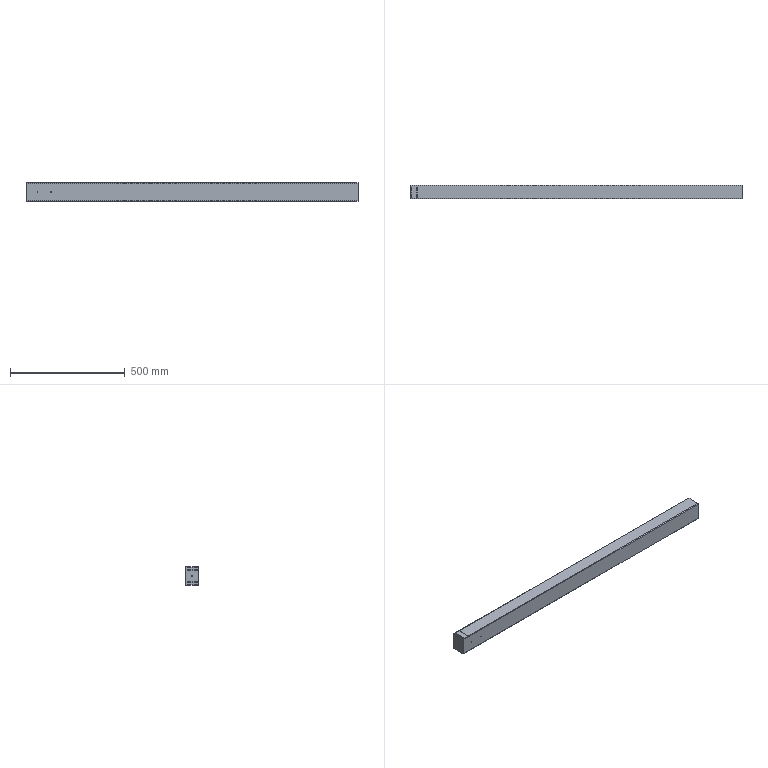Part | NX | 1 solid | 55 faces | box 1446 x 60 x 80 mm | volume 2283808 mm3 | cylinder 33 | plane 12 | cone 10 | commonest cylinder face diameters 3.3 x20 5.236 x8 4.2 x5
STEP:
#1=CARTESIAN_POINT('',(1126.,565.,37.382));
#2=VERTEX_POINT('',#1);
#3=CARTESIAN_POINT('',(-320.,565.,37.382));
#4=VERTEX_POINT('',#3);
#5=CARTESIAN_POINT('',(1126.,565.,37.382));
#6=DIRECTION('',(-1.,0.,0.));
#7=VECTOR('',#6,1000.);
#8=LINE('',#5,#7);
#9=EDGE_CURVE('',#2,#4,#8,.T.);
#10=ORIENTED_EDGE('',*,*,#9,.T.);
#11=CARTESIAN_POINT('',(-320.,562.382,40.));
#12=VERTEX_POINT('',#11);
#13=CARTESIAN_POINT('',(-320.,562.382,37.382));
#14=DIRECTION('',(1.,0.,0.));
#15=DIRECTION('',(0.,0.,1.));
#16=AXIS2_PLACEMENT_3D('',#13,#14,#15);
#17=CIRCLE('',#16,2.618);
#18=EDGE_CURVE('',#4,#12,#17,.T.);
#19=ORIENTED_EDGE('',*,*,#18,.T.);
#20=CARTESIAN_POINT('',(1126.,562.382,40.));
#21=VERTEX_POINT('',#20);
#22=CARTESIAN_POINT('',(1126.,562.382,40.));
#23=DIRECTION('',(-1.,0.,0.));
#24=VECTOR('',#23,1000.);
#25=LINE('',#22,#24);
#26=EDGE_CURVE('',#21,#12,#25,.T.);
#27=ORIENTED_EDGE('',*,*,#26,.F.);
#28=CARTESIAN_POINT('',(1126.,562.382,37.382));
#29=DIRECTION('',(1.,0.,0.));
#30=DIRECTION('',(0.,0.,1.));
#31=AXIS2_PLACEMENT_3D('',#28,#29,#30);
#32=CIRCLE('',#31,2.618);
#33=EDGE_CURVE('',#2,#21,#32,.T.);
#34=ORIENTED_EDGE('',*,*,#33,.F.);
#35=EDGE_LOOP('',(#10,#19,#27,#34));
#36=FACE_BOUND('',#35,.T.);
#37=CARTESIAN_POINT('',(1126.,562.382,37.382));
#38=DIRECTION('',(-1.,0.,0.));
#39=DIRECTION('',(0.,0.,1.));
#40=AXIS2_PLACEMENT_3D('',#37,#38,#39);
#41=CYLINDRICAL_SURFACE('',#40,2.618);
#42=ADVANCED_FACE('',(#36),#41,.T.);
#43=CARTESIAN_POINT('',(-289.5,551.35,40.));
#44=VERTEX_POINT('',#43);
#45=CARTESIAN_POINT('',(-289.5,553.,40.));
#46=DIRECTION('',(0.,0.,1.));
#47=DIRECTION('',(0.,-1.,0.));
#48=AXIS2_PLACEMENT_3D('',#45,#46,#47);
#49=CIRCLE('',#48,1.65);
#50=EDGE_CURVE('',#44,#44,#49,.T.);
#51=ORIENTED_EDGE('',*,*,#50,.F.);
#52=EDGE_LOOP('',(#51));
#53=FACE_BOUND('',#52,.T.);
#54=CARTESIAN_POINT('',(-314.5,551.35,40.));
#55=VERTEX_POINT('',#54);
#56=CARTESIAN_POINT('',(-314.5,553.,40.));
#57=DIRECTION('',(0.,0.,1.));
#58=DIRECTION('',(0.,-1.,0.));
#59=AXIS2_PLACEMENT_3D('',#56,#57,#58);
#60=CIRCLE('',#59,1.65);
#61=EDGE_CURVE('',#55,#55,#60,.T.);
#62=ORIENTED_EDGE('',*,*,#61,.F.);
#63=EDGE_LOOP('',(#62));
#64=FACE_BOUND('',#63,.T.);
#65=CARTESIAN_POINT('',(-289.5,541.35,40.));
#66=VERTEX_POINT('',#65);
#67=CARTESIAN_POINT('',(-289.5,543.,40.));
#68=DIRECTION('',(0.,0.,1.));
#69=DIRECTION('',(0.,-1.,0.));
#70=AXIS2_PLACEMENT_3D('',#67,#68,#69);
#71=CIRCLE('',#70,1.65);
#72=EDGE_CURVE('',#66,#66,#71,.T.);
#73=ORIENTED_EDGE('',*,*,#72,.F.);
#74=EDGE_LOOP('',(#73));
#75=FACE_BOUND('',#74,.T.);
#76=CARTESIAN_POINT('',(-314.5,541.35,40.));
#77=VERTEX_POINT('',#76);
#78=CARTESIAN_POINT('',(-314.5,543.,40.));
#79=DIRECTION('',(0.,0.,1.));
#80=DIRECTION('',(0.,-1.,0.));
#81=AXIS2_PLACEMENT_3D('',#78,#79,#80);
#82=CIRCLE('',#81,1.65);
#83=EDGE_CURVE('',#77,#77,#82,.T.);
#84=ORIENTED_EDGE('',*,*,#83,.F.);
#85=EDGE_LOOP('',(#84));
#86=FACE_BOUND('',#85,.T.);
#87=CARTESIAN_POINT('',(-289.5,531.35,40.));
#88=VERTEX_POINT('',#87);
#89=CARTESIAN_POINT('',(-289.5,533.,40.));
#90=DIRECTION('',(0.,0.,1.));
#91=DIRECTION('',(0.,-1.,0.));
#92=AXIS2_PLACEMENT_3D('',#89,#90,#91);
#93=CIRCLE('',#92,1.65);
#94=EDGE_CURVE('',#88,#88,#93,.T.);
#95=ORIENTED_EDGE('',*,*,#94,.F.);
#96=EDGE_LOOP('',(#95));
#97=FACE_BOUND('',#96,.T.);
#98=CARTESIAN_POINT('',(-314.5,531.35,40.));
#99=VERTEX_POINT('',#98);
#100=CARTESIAN_POINT('',(-314.5,533.,40.));
#101=DIRECTION('',(0.,0.,1.));
#102=DIRECTION('',(0.,-1.,0.));
#103=AXIS2_PLACEMENT_3D('',#100,#101,#102);
#104=CIRCLE('',#103,1.65);
#105=EDGE_CURVE('',#99,#99,#104,.T.);
#106=ORIENTED_EDGE('',*,*,#105,.F.);
#107=EDGE_LOOP('',(#106));
#108=FACE_BOUND('',#107,.T.);
#109=CARTESIAN_POINT('',(-289.5,521.35,40.));
#110=VERTEX_POINT('',#109);
#111=CARTESIAN_POINT('',(-289.5,523.,40.));
#112=DIRECTION('',(0.,0.,1.));
#113=DIRECTION('',(0.,-1.,0.));
#114=AXIS2_PLACEMENT_3D('',#111,#112,#113);
#115=CIRCLE('',#114,1.65);
#116=EDGE_CURVE('',#110,#110,#115,.T.);
#117=ORIENTED_EDGE('',*,*,#116,.F.);
#118=EDGE_LOOP('',(#117));
#119=FACE_BOUND('',#118,.T.);
#120=CARTESIAN_POINT('',(-314.5,521.35,40.));
#121=VERTEX_POINT('',#120);
#122=CARTESIAN_POINT('',(-314.5,523.,40.));
#123=DIRECTION('',(0.,0.,1.));
#124=DIRECTION('',(0.,-1.,0.));
#125=AXIS2_PLACEMENT_3D('',#122,#123,#124);
#126=CIRCLE('',#125,1.65);
#127=EDGE_CURVE('',#121,#121,#126,.T.);
#128=ORIENTED_EDGE('',*,*,#127,.F.);
#129=EDGE_LOOP('',(#128));
#130=FACE_BOUND('',#129,.T.);
#131=CARTESIAN_POINT('',(-289.5,511.35,40.));
#132=VERTEX_POINT('',#131);
#133=CARTESIAN_POINT('',(-289.5,513.,40.));
#134=DIRECTION('',(0.,0.,1.));
#135=DIRECTION('',(0.,-1.,0.));
#136=AXIS2_PLACEMENT_3D('',#133,#134,#135);
#137=CIRCLE('',#136,1.65);
#138=EDGE_CURVE('',#132,#132,#137,.T.);
#139=ORIENTED_EDGE('',*,*,#138,.F.);
#140=EDGE_LOOP('',(#139));
#141=FACE_BOUND('',#140,.T.);
#142=CARTESIAN_POINT('',(-314.5,511.35,40.));
#143=VERTEX_POINT('',#142);
#144=CARTESIAN_POINT('',(-314.5,513.,40.));
#145=DIRECTION('',(0.,0.,1.));
#146=DIRECTION('',(0.,-1.,0.));
#147=AXIS2_PLACEMENT_3D('',#144,#145,#146);
#148=CIRCLE('',#147,1.65);
#149=EDGE_CURVE('',#143,#143,#148,.T.);
#150=ORIENTED_EDGE('',*,*,#149,.F.);
#151=EDGE_LOOP('',(#150));
#152=FACE_BOUND('',#151,.T.);
#153=ORIENTED_EDGE('',*,*,#26,.T.);
#154=CARTESIAN_POINT('',(-320.,507.618,40.));
#155=VERTEX_POINT('',#154);
#156=CARTESIAN_POINT('',(-320.,507.618,40.));
#157=DIRECTION('',(0.,-1.,0.));
#158=VECTOR('',#157,1000.);
#159=LINE('',#156,#158);
#160=EDGE_CURVE('',#12,#155,#159,.T.);
#161=ORIENTED_EDGE('',*,*,#160,.T.);
#162=CARTESIAN_POINT('',(1126.,507.618,40.));
#163=VERTEX_POINT('',#162);
#164=CARTESIAN_POINT('',(1126.,507.618,40.));
#165=DIRECTION('',(-1.,0.,0.));
#166=VECTOR('',#165,1000.);
#167=LINE('',#164,#166);
#168=EDGE_CURVE('',#163,#155,#167,.T.);
#169=ORIENTED_EDGE('',*,*,#168,.F.);
#170=CARTESIAN_POINT('',(1126.,507.618,40.));
#171=DIRECTION('',(0.,-1.,0.));
#172=VECTOR('',#171,1000.);
#173=LINE('',#170,#172);
#174=EDGE_CURVE('',#21,#163,#173,.T.);
#175=ORIENTED_EDGE('',*,*,#174,.F.);
#176=EDGE_LOOP('',(#153,#161,#169,#175));
#177=FACE_BOUND('',#176,.T.);
#178=CARTESIAN_POINT('',(1126.,507.618,40.));
#179=DIRECTION('',(0.,0.,-1.));
#180=DIRECTION('',(0.,1.,0.));
#181=AXIS2_PLACEMENT_3D('',#178,#179,#180);
#182=PLANE('',#181);
#183=ADVANCED_FACE('',(#53,#64,#75,#86,#97,#108,#119,#130,#141,#152,#177),#182,.F.);
#184=ORIENTED_EDGE('',*,*,#168,.T.);
#185=CARTESIAN_POINT('',(-320.,505.,37.382));
#186=VERTEX_POINT('',#185);
#187=CARTESIAN_POINT('',(-320.,507.618,37.382));
#188=DIRECTION('',(1.,0.,0.));
#189=DIRECTION('',(0.,0.,-1.));
#190=AXIS2_PLACEMENT_3D('',#187,#188,#189);
#191=CIRCLE('',#190,2.618);
#192=EDGE_CURVE('',#155,#186,#191,.T.);
#193=ORIENTED_EDGE('',*,*,#192,.T.);
#194=CARTESIAN_POINT('',(1126.,505.,37.382));
#195=VERTEX_POINT('',#194);
#196=CARTESIAN_POINT('',(1126.,505.,37.382));
#197=DIRECTION('',(-1.,0.,0.));
#198=VECTOR('',#197,1000.);
#199=LINE('',#196,#198);
#200=EDGE_CURVE('',#195,#186,#199,.T.);
#201=ORIENTED_EDGE('',*,*,#200,.F.);
#202=CARTESIAN_POINT('',(1126.,507.618,37.382));
#203=DIRECTION('',(1.,0.,0.));
#204=DIRECTION('',(0.,0.,-1.));
#205=AXIS2_PLACEMENT_3D('',#202,#203,#204);
#206=CIRCLE('',#205,2.618);
#207=EDGE_CURVE('',#163,#195,#206,.T.);
#208=ORIENTED_EDGE('',*,*,#207,.F.);
#209=EDGE_LOOP('',(#184,#193,#201,#208));
#210=FACE_BOUND('',#209,.T.);
#211=CARTESIAN_POINT('',(1126.,507.618,37.382));
#212=DIRECTION('',(-1.,0.,0.));
#213=DIRECTION('',(0.,0.,1.));
#214=AXIS2_PLACEMENT_3D('',#211,#212,#213);
#215=CYLINDRICAL_SURFACE('',#214,2.618);
#216=ADVANCED_FACE('',(#210),#215,.T.);
#217=CARTESIAN_POINT('',(-212.426,505.,-2.1));
#218=VERTEX_POINT('',#217);
#219=CARTESIAN_POINT('',(-212.426,505.,0.));
#220=DIRECTION('',(0.,-1.,0.));
#221=DIRECTION('',(0.,0.,-1.));
#222=AXIS2_PLACEMENT_3D('',#219,#220,#221);
#223=CIRCLE('',#222,2.1);
#224=EDGE_CURVE('',#218,#218,#223,.T.);
#225=ORIENTED_EDGE('',*,*,#224,.F.);
#226=EDGE_LOOP('',(#225));
#227=FACE_BOUND('',#226,.T.);
#228=CARTESIAN_POINT('',(-270.,505.,-2.1));
#229=VERTEX_POINT('',#228);
#230=CARTESIAN_POINT('',(-270.,505.,0.));
#231=DIRECTION('',(0.,-1.,0.));
#232=DIRECTION('',(0.,0.,-1.));
#233=AXIS2_PLACEMENT_3D('',#230,#231,#232);
#234=CIRCLE('',#233,2.1);
#235=EDGE_CURVE('',#229,#229,#234,.T.);
#236=ORIENTED_EDGE('',*,*,#235,.F.);
#237=EDGE_LOOP('',(#236));
#238=FACE_BOUND('',#237,.T.);
#239=ORIENTED_EDGE('',*,*,#200,.T.);
#240=CARTESIAN_POINT('',(-320.,505.,-37.382));
#241=VERTEX_POINT('',#240);
#242=CARTESIAN_POINT('',(-320.,505.,37.382));
#243=DIRECTION('',(0.,0.,-1.));
#244=VECTOR('',#243,1000.);
#245=LINE('',#242,#244);
#246=EDGE_CURVE('',#186,#241,#245,.T.);
#247=ORIENTED_EDGE('',*,*,#246,.T.);
#248=CARTESIAN_POINT('',(1126.,505.,-37.382));
#249=VERTEX_POINT('',#248);
#250=CARTESIAN_POINT('',(1126.,505.,-37.382));
#251=DIRECTION('',(-1.,0.,0.));
#252=VECTOR('',#251,1000.);
#253=LINE('',#250,#252);
#254=EDGE_CURVE('',#249,#241,#253,.T.);
#255=ORIENTED_EDGE('',*,*,#254,.F.);
#256=CARTESIAN_POINT('',(1126.,505.,37.382));
#257=DIRECTION('',(0.,0.,-1.));
#258=VECTOR('',#257,1000.);
#259=LINE('',#256,#258);
#260=EDGE_CURVE('',#195,#249,#259,.T.);
#261=ORIENTED_EDGE('',*,*,#260,.F.);
#262=EDGE_LOOP('',(#239,#247,#255,#261));
#263=FACE_BOUND('',#262,.T.);
#264=CARTESIAN_POINT('',(1126.,505.,37.382));
#265=DIRECTION('',(0.,1.,0.));
#266=DIRECTION('',(0.,0.,1.));
#267=AXIS2_PLACEMENT_3D('',#264,#265,#266);
#268=PLANE('',#267);
#269=ADVANCED_FACE('',(#227,#238,#263),#268,.F.);
#270=ORIENTED_EDGE('',*,*,#254,.T.);
#271=CARTESIAN_POINT('',(-320.,507.618,-40.));
#272=VERTEX_POINT('',#271);
#273=CARTESIAN_POINT('',(-320.,507.618,-37.382));
#274=DIRECTION('',(1.,0.,0.));
#275=DIRECTION('',(0.,0.,-1.));
#276=AXIS2_PLACEMENT_3D('',#273,#274,#275);
#277=CIRCLE('',#276,2.618);
#278=EDGE_CURVE('',#241,#272,#277,.T.);
#279=ORIENTED_EDGE('',*,*,#278,.T.);
#280=CARTESIAN_POINT('',(1126.,507.618,-40.));
#281=VERTEX_POINT('',#280);
#282=CARTESIAN_POINT('',(1126.,507.618,-40.));
#283=DIRECTION('',(-1.,0.,0.));
#284=VECTOR('',#283,1000.);
#285=LINE('',#282,#284);
#286=EDGE_CURVE('',#281,#272,#285,.T.);
#287=ORIENTED_EDGE('',*,*,#286,.F.);
#288=CARTESIAN_POINT('',(1126.,507.618,-37.382));
#289=DIRECTION('',(1.,0.,0.));
#290=DIRECTION('',(0.,0.,-1.));
#291=AXIS2_PLACEMENT_3D('',#288,#289,#290);
#292=CIRCLE('',#291,2.618);
#293=EDGE_CURVE('',#249,#281,#292,.T.);
#294=ORIENTED_EDGE('',*,*,#293,.F.);
#295=EDGE_LOOP('',(#270,#279,#287,#294));
#296=FACE_BOUND('',#295,.T.);
#297=CARTESIAN_POINT('',(1126.,507.618,-37.382));
#298=DIRECTION('',(-1.,0.,0.));
#299=DIRECTION('',(0.,0.,1.));
#300=AXIS2_PLACEMENT_3D('',#297,#298,#299);
#301=CYLINDRICAL_SURFACE('',#300,2.618);
#302=ADVANCED_FACE('',(#296),#301,.T.);
#303=CARTESIAN_POINT('',(-289.5,554.65,-40.));
#304=VERTEX_POINT('',#303);
#305=CARTESIAN_POINT('',(-289.5,553.,-40.));
#306=DIRECTION('',(0.,0.,-1.));
#307=DIRECTION('',(0.,1.,0.));
#308=AXIS2_PLACEMENT_3D('',#305,#306,#307);
#309=CIRCLE('',#308,1.65);
#310=EDGE_CURVE('',#304,#304,#309,.T.);
#311=ORIENTED_EDGE('',*,*,#310,.F.);
#312=EDGE_LOOP('',(#311));
#313=FACE_BOUND('',#312,.T.);
#314=CARTESIAN_POINT('',(-314.5,554.65,-40.));
#315=VERTEX_POINT('',#314);
#316=CARTESIAN_POINT('',(-314.5,553.,-40.));
#317=DIRECTION('',(0.,0.,-1.));
#318=DIRECTION('',(0.,1.,0.));
#319=AXIS2_PLACEMENT_3D('',#316,#317,#318);
#320=CIRCLE('',#319,1.65);
#321=EDGE_CURVE('',#315,#315,#320,.T.);
#322=ORIENTED_EDGE('',*,*,#321,.F.);
#323=EDGE_LOOP('',(#322));
#324=FACE_BOUND('',#323,.T.);
#325=CARTESIAN_POINT('',(-289.5,544.65,-40.));
#326=VERTEX_POINT('',#325);
#327=CARTESIAN_POINT('',(-289.5,543.,-40.));
#328=DIRECTION('',(0.,0.,-1.));
#329=DIRECTION('',(0.,1.,0.));
#330=AXIS2_PLACEMENT_3D('',#327,#328,#329);
#331=CIRCLE('',#330,1.65);
#332=EDGE_CURVE('',#326,#326,#331,.T.);
#333=ORIENTED_EDGE('',*,*,#332,.F.);
#334=EDGE_LOOP('',(#333));
#335=FACE_BOUND('',#334,.T.);
#336=CARTESIAN_POINT('',(-314.5,544.65,-40.));
#337=VERTEX_POINT('',#336);
#338=CARTESIAN_POINT('',(-314.5,543.,-40.));
#339=DIRECTION('',(0.,0.,-1.));
#340=DIRECTION('',(0.,1.,0.));
#341=AXIS2_PLACEMENT_3D('',#338,#339,#340);
#342=CIRCLE('',#341,1.65);
#343=EDGE_CURVE('',#337,#337,#342,.T.);
#344=ORIENTED_EDGE('',*,*,#343,.F.);
#345=EDGE_LOOP('',(#344));
#346=FACE_BOUND('',#345,.T.);
#347=CARTESIAN_POINT('',(-289.5,534.65,-40.));
#348=VERTEX_POINT('',#347);
#349=CARTESIAN_POINT('',(-289.5,533.,-40.));
#350=DIRECTION('',(0.,0.,-1.));
#351=DIRECTION('',(0.,1.,0.));
#352=AXIS2_PLACEMENT_3D('',#349,#350,#351);
#353=CIRCLE('',#352,1.65);
#354=EDGE_CURVE('',#348,#348,#353,.T.);
#355=ORIENTED_EDGE('',*,*,#354,.F.);
#356=EDGE_LOOP('',(#355));
#357=FACE_BOUND('',#356,.T.);
#358=CARTESIAN_POINT('',(-314.5,534.65,-40.));
#359=VERTEX_POINT('',#358);
#360=CARTESIAN_POINT('',(-314.5,533.,-40.));
#361=DIRECTION('',(0.,0.,-1.));
#362=DIRECTION('',(0.,1.,0.));
#363=AXIS2_PLACEMENT_3D('',#360,#361,#362);
#364=CIRCLE('',#363,1.65);
#365=EDGE_CURVE('',#359,#359,#364,.T.);
#366=ORIENTED_EDGE('',*,*,#365,.F.);
#367=EDGE_LOOP('',(#366));
#368=FACE_BOUND('',#367,.T.);
#369=CARTESIAN_POINT('',(-289.5,524.65,-40.));
#370=VERTEX_POINT('',#369);
#371=CARTESIAN_POINT('',(-289.5,523.,-40.));
#372=DIRECTION('',(0.,0.,-1.));
#373=DIRECTION('',(0.,1.,0.));
#374=AXIS2_PLACEMENT_3D('',#371,#372,#373);
#375=CIRCLE('',#374,1.65);
#376=EDGE_CURVE('',#370,#370,#375,.T.);
#377=ORIENTED_EDGE('',*,*,#376,.F.);
#378=EDGE_LOOP('',(#377));
#379=FACE_BOUND('',#378,.T.);
#380=CARTESIAN_POINT('',(-314.5,524.65,-40.));
#381=VERTEX_POINT('',#380);
#382=CARTESIAN_POINT('',(-314.5,523.,-40.));
#383=DIRECTION('',(0.,0.,-1.));
#384=DIRECTION('',(0.,1.,0.));
#385=AXIS2_PLACEMENT_3D('',#382,#383,#384);
#386=CIRCLE('',#385,1.65);
#387=EDGE_CURVE('',#381,#381,#386,.T.);
#388=ORIENTED_EDGE('',*,*,#387,.F.);
#389=EDGE_LOOP('',(#388));
#390=FACE_BOUND('',#389,.T.);
#391=CARTESIAN_POINT('',(-289.5,514.65,-40.));
#392=VERTEX_POINT('',#391);
#393=CARTESIAN_POINT('',(-289.5,513.,-40.));
#394=DIRECTION('',(0.,0.,-1.));
#395=DIRECTION('',(0.,1.,0.));
#396=AXIS2_PLACEMENT_3D('',#393,#394,#395);
#397=CIRCLE('',#396,1.65);
#398=EDGE_CURVE('',#392,#392,#397,.T.);
#399=ORIENTED_EDGE('',*,*,#398,.F.);
#400=EDGE_LOOP('',(#399));
#401=FACE_BOUND('',#400,.T.);
#402=CARTESIAN_POINT('',(-314.5,514.65,-40.));
#403=VERTEX_POINT('',#402);
#404=CARTESIAN_POINT('',(-314.5,513.,-40.));
#405=DIRECTION('',(0.,0.,-1.));
#406=DIRECTION('',(0.,1.,0.));
#407=AXIS2_PLACEMENT_3D('',#404,#405,#406);
#408=CIRCLE('',#407,1.65);
#409=EDGE_CURVE('',#403,#403,#408,.T.);
#410=ORIENTED_EDGE('',*,*,#409,.F.);
#411=EDGE_LOOP('',(#410));
#412=FACE_BOUND('',#411,.T.);
#413=ORIENTED_EDGE('',*,*,#286,.T.);
#414=CARTESIAN_POINT('',(-320.,562.382,-40.));
#415=VERTEX_POINT('',#414);
#416=CARTESIAN_POINT('',(-320.,507.618,-40.));
#417=DIRECTION('',(0.,1.,0.));
#418=VECTOR('',#417,1000.);
#419=LINE('',#416,#418);
#420=EDGE_CURVE('',#272,#415,#419,.T.);
#421=ORIENTED_EDGE('',*,*,#420,.T.);
#422=CARTESIAN_POINT('',(1126.,562.382,-40.));
#423=VERTEX_POINT('',#422);
#424=CARTESIAN_POINT('',(1126.,562.382,-40.));
#425=DIRECTION('',(-1.,0.,0.));
#426=VECTOR('',#425,1000.);
#427=LINE('',#424,#426);
#428=EDGE_CURVE('',#423,#415,#427,.T.);
#429=ORIENTED_EDGE('',*,*,#428,.F.);
#430=CARTESIAN_POINT('',(1126.,507.618,-40.));
#431=DIRECTION('',(0.,1.,0.));
#432=VECTOR('',#431,1000.);
#433=LINE('',#430,#432);
#434=EDGE_CURVE('',#281,#423,#433,.T.);
#435=ORIENTED_EDGE('',*,*,#434,.F.);
#436=EDGE_LOOP('',(#413,#421,#429,#435));
#437=FACE_BOUND('',#436,.T.);
#438=CARTESIAN_POINT('',(1126.,507.618,-40.));
#439=DIRECTION('',(0.,0.,1.));
#440=DIRECTION('',(0.,-1.,0.));
#441=AXIS2_PLACEMENT_3D('',#438,#439,#440);
#442=PLANE('',#441);
#443=ADVANCED_FACE('',(#313,#324,#335,#346,#357,#368,#379,#390,#401,#412,#437),#442,.F.);
#444=ORIENTED_EDGE('',*,*,#428,.T.);
#445=CARTESIAN_POINT('',(-320.,565.,-37.382));
#446=VERTEX_POINT('',#445);
#447=CARTESIAN_POINT('',(-320.,562.382,-37.382));
#448=DIRECTION('',(1.,0.,0.));
#449=DIRECTION('',(0.,0.,-1.));
#450=AXIS2_PLACEMENT_3D('',#447,#448,#449);
#451=CIRCLE('',#450,2.618);
#452=EDGE_CURVE('',#415,#446,#451,.T.);
#453=ORIENTED_EDGE('',*,*,#452,.T.);
#454=CARTESIAN_POINT('',(1126.,565.,-37.382));
#455=VERTEX_POINT('',#454);
#456=CARTESIAN_POINT('',(1126.,565.,-37.382));
#457=DIRECTION('',(-1.,0.,0.));
#458=VECTOR('',#457,1000.);
#459=LINE('',#456,#458);
#460=EDGE_CURVE('',#455,#446,#459,.T.);
#461=ORIENTED_EDGE('',*,*,#460,.F.);
#462=CARTESIAN_POINT('',(1126.,562.382,-37.382));
#463=DIRECTION('',(1.,0.,0.));
#464=DIRECTION('',(0.,0.,-1.));
#465=AXIS2_PLACEMENT_3D('',#462,#463,#464);
#466=CIRCLE('',#465,2.618);
#467=EDGE_CURVE('',#423,#455,#466,.T.);
#468=ORIENTED_EDGE('',*,*,#467,.F.);
#469=EDGE_LOOP('',(#444,#453,#461,#468));
#470=FACE_BOUND('',#469,.T.);
#471=CARTESIAN_POINT('',(1126.,562.382,-37.382));
#472=DIRECTION('',(-1.,0.,0.));
#473=DIRECTION('',(0.,0.,1.));
#474=AXIS2_PLACEMENT_3D('',#471,#472,#473);
#475=CYLINDRICAL_SURFACE('',#474,2.618);
#476=ADVANCED_FACE('',(#470),#475,.T.);
#477=ORIENTED_EDGE('',*,*,#460,.T.);
#478=CARTESIAN_POINT('',(-320.,565.,37.382));
#479=DIRECTION('',(0.,0.,1.));
#480=VECTOR('',#479,1000.);
#481=LINE('',#478,#480);
#482=EDGE_CURVE('',#446,#4,#481,.T.);
#483=ORIENTED_EDGE('',*,*,#482,.T.);
#484=ORIENTED_EDGE('',*,*,#9,.F.);
#485=CARTESIAN_POINT('',(1126.,565.,37.382));
#486=DIRECTION('',(0.,0.,1.));
#487=VECTOR('',#486,1000.);
#488=LINE('',#485,#487);
#489=EDGE_CURVE('',#455,#2,#488,.T.);
#490=ORIENTED_EDGE('',*,*,#489,.F.);
#491=EDGE_LOOP('',(#477,#483,#484,#490));
#492=FACE_BOUND('',#491,.T.);
#493=CARTESIAN_POINT('',(1126.,565.,37.382));
#494=DIRECTION('',(0.,-1.,0.));
#495=DIRECTION('',(0.,0.,-1.));
#496=AXIS2_PLACEMENT_3D('',#493,#494,#495);
#497=PLANE('',#496);
#498=ADVANCED_FACE('',(#492),#497,.F.);
#499=CARTESIAN_POINT('',(1126.,552.5,5.9));
#500=VERTEX_POINT('',#499);
#501=CARTESIAN_POINT('',(1126.,552.5,8.));
#502=DIRECTION('',(1.,0.,0.));
#503=DIRECTION('',(0.,0.,-1.));
#504=AXIS2_PLACEMENT_3D('',#501,#502,#503);
#505=CIRCLE('',#504,2.1);
#506=EDGE_CURVE('',#500,#500,#505,.T.);
#507=ORIENTED_EDGE('',*,*,#506,.F.);
#508=EDGE_LOOP('',(#507));
#509=FACE_BOUND('',#508,.T.);
#510=CARTESIAN_POINT('',(1126.,552.5,-24.1));
#511=VERTEX_POINT('',#510);
#512=CARTESIAN_POINT('',(1126.,552.5,-22.));
#513=DIRECTION('',(1.,0.,0.));
#514=DIRECTION('',(0.,0.,-1.));
#515=AXIS2_PLACEMENT_3D('',#512,#513,#514);
#516=CIRCLE('',#515,2.1);
#517=EDGE_CURVE('',#511,#511,#516,.T.);
#518=ORIENTED_EDGE('',*,*,#517,.F.);
#519=EDGE_LOOP('',(#518));
#520=FACE_BOUND('',#519,.T.);
#521=ORIENTED_EDGE('',*,*,#33,.T.);
#522=ORIENTED_EDGE('',*,*,#174,.T.);
#523=ORIENTED_EDGE('',*,*,#207,.T.);
#524=ORIENTED_EDGE('',*,*,#260,.T.);
#525=ORIENTED_EDGE('',*,*,#293,.T.);
#526=ORIENTED_EDGE('',*,*,#434,.T.);
#527=ORIENTED_EDGE('',*,*,#467,.T.);
#528=ORIENTED_EDGE('',*,*,#489,.T.);
#529=EDGE_LOOP('',(#521,#522,#523,#524,#525,#526,#527,#528));
#530=FACE_BOUND('',#529,.T.);
#531=CARTESIAN_POINT('',(1126.,562.382,37.382));
#532=DIRECTION('',(-1.,0.,0.));
#533=DIRECTION('',(0.,0.,1.));
#534=AXIS2_PLACEMENT_3D('',#531,#532,#533);
#535=PLANE('',#534);
#536=ADVANCED_FACE('',(#509,#520,#530),#535,.F.);
#537=CARTESIAN_POINT('',(-320.,537.1,0.));
#538=VERTEX_POINT('',#537);
#539=CARTESIAN_POINT('',(-320.,535.,0.));
#540=DIRECTION('',(-1.,0.,0.));
#541=DIRECTION('',(0.,1.,0.));
#542=AXIS2_PLACEMENT_3D('',#539,#540,#541);
#543=CIRCLE('',#542,2.1);
#544=EDGE_CURVE('',#538,#538,#543,.T.);
#545=ORIENTED_EDGE('',*,*,#544,.F.);
#546=EDGE_LOOP('',(#545));
#547=FACE_BOUND('',#546,.T.);
#548=ORIENTED_EDGE('',*,*,#18,.F.);
#549=ORIENTED_EDGE('',*,*,#482,.F.);
#550=ORIENTED_EDGE('',*,*,#452,.F.);
#551=ORIENTED_EDGE('',*,*,#420,.F.);
#552=ORIENTED_EDGE('',*,*,#278,.F.);
#553=ORIENTED_EDGE('',*,*,#246,.F.);
#554=ORIENTED_EDGE('',*,*,#192,.F.);
#555=ORIENTED_EDGE('',*,*,#160,.F.);
#556=EDGE_LOOP('',(#548,#549,#550,#551,#552,#553,#554,#555));
#557=FACE_BOUND('',#556,.T.);
#558=CARTESIAN_POINT('',(-320.,562.382,37.382));
#559=DIRECTION('',(-1.,0.,0.));
#560=DIRECTION('',(0.,0.,1.));
#561=AXIS2_PLACEMENT_3D('',#558,#559,#560);
#562=PLANE('',#561);
#563=ADVANCED_FACE('',(#547,#557),#562,.T.);
#564=ORIENTED_EDGE('',*,*,#517,.T.);
#565=EDGE_LOOP('',(#564));
#566=FACE_BOUND('',#565,.T.);
#567=CARTESIAN_POINT('',(1116.,552.5,-24.1));
#568=VERTEX_POINT('',#567);
#569=CARTESIAN_POINT('',(1116.,552.5,-22.));
#570=DIRECTION('',(1.,0.,0.));
#571=DIRECTION('',(0.,0.,-1.));
#572=AXIS2_PLACEMENT_3D('',#569,#570,#571);
#573=CIRCLE('',#572,2.1);
#574=EDGE_CURVE('',#568,#568,#573,.T.);
#575=ORIENTED_EDGE('',*,*,#574,.F.);
#576=EDGE_LOOP('',(#575));
#577=FACE_BOUND('',#576,.T.);
#578=CARTESIAN_POINT('',(1126.,552.5,-22.));
#579=DIRECTION('',(1.,0.,0.));
#580=DIRECTION('',(0.,0.,-1.));
#581=AXIS2_PLACEMENT_3D('',#578,#579,#580);
#582=CYLINDRICAL_SURFACE('',#581,2.1);
#583=ADVANCED_FACE('',(#566,#577),#582,.F.);
#584=CARTESIAN_POINT('',(-310.,535.,2.1));
#585=VERTEX_POINT('',#584);
#586=CARTESIAN_POINT('',(-310.,535.,0.));
#587=DIRECTION('',(-1.,0.,0.));
#588=DIRECTION('',(0.,0.,1.));
#589=AXIS2_PLACEMENT_3D('',#586,#587,#588);
#590=CIRCLE('',#589,2.1);
#591=EDGE_CURVE('',#585,#585,#590,.T.);
#592=ORIENTED_EDGE('',*,*,#591,.T.);
#593=EDGE_LOOP('',(#592));
#594=FACE_BOUND('',#593,.T.);
#595=CARTESIAN_POINT('',(-310.,513.618,-34.));
#596=VERTEX_POINT('',#595);
#597=CARTESIAN_POINT('',(-310.,511.,-31.382));
#598=VERTEX_POINT('',#597);
#599=CARTESIAN_POINT('',(-310.,513.618,-31.382));
#600=DIRECTION('',(-1.,0.,0.));
#601=DIRECTION('',(0.,0.,1.));
#602=AXIS2_PLACEMENT_3D('',#599,#600,#601);
#603=CIRCLE('',#602,2.618);
#604=EDGE_CURVE('',#596,#598,#603,.T.);
#605=ORIENTED_EDGE('',*,*,#604,.F.);
#606=CARTESIAN_POINT('',(-310.,556.382,-34.));
#607=VERTEX_POINT('',#606);
#608=CARTESIAN_POINT('',(-310.,513.618,-34.));
#609=DIRECTION('',(0.,-1.,0.));
#610=VECTOR('',#609,1000.);
#611=LINE('',#608,#610);
#612=EDGE_CURVE('',#607,#596,#611,.T.);
#613=ORIENTED_EDGE('',*,*,#612,.F.);
#614=CARTESIAN_POINT('',(-310.,559.,-31.382));
#615=VERTEX_POINT('',#614);
#616=CARTESIAN_POINT('',(-310.,556.382,-31.382));
#617=DIRECTION('',(-1.,0.,0.));
#618=DIRECTION('',(0.,0.,1.));
#619=AXIS2_PLACEMENT_3D('',#616,#617,#618);
#620=CIRCLE('',#619,2.618);
#621=EDGE_CURVE('',#615,#607,#620,.T.);
#622=ORIENTED_EDGE('',*,*,#621,.F.);
#623=CARTESIAN_POINT('',(-310.,559.,31.382));
#624=VERTEX_POINT('',#623);
#625=CARTESIAN_POINT('',(-310.,559.,31.382));
#626=DIRECTION('',(0.,0.,-1.));
#627=VECTOR('',#626,1000.);
#628=LINE('',#625,#627);
#629=EDGE_CURVE('',#624,#615,#628,.T.);
#630=ORIENTED_EDGE('',*,*,#629,.F.);
#631=CARTESIAN_POINT('',(-310.,556.382,34.));
#632=VERTEX_POINT('',#631);
#633=CARTESIAN_POINT('',(-310.,556.382,31.382));
#634=DIRECTION('',(-1.,0.,0.));
#635=DIRECTION('',(0.,0.,1.));
#636=AXIS2_PLACEMENT_3D('',#633,#634,#635);
#637=CIRCLE('',#636,2.618);
#638=EDGE_CURVE('',#632,#624,#637,.T.);
#639=ORIENTED_EDGE('',*,*,#638,.F.);
#640=CARTESIAN_POINT('',(-310.,513.618,34.));
#641=VERTEX_POINT('',#640);
#642=CARTESIAN_POINT('',(-310.,513.618,34.));
#643=DIRECTION('',(0.,1.,0.));
#644=VECTOR('',#643,1000.);
#645=LINE('',#642,#644);
#646=EDGE_CURVE('',#641,#632,#645,.T.);
#647=ORIENTED_EDGE('',*,*,#646,.F.);
#648=CARTESIAN_POINT('',(-310.,511.,31.382));
#649=VERTEX_POINT('',#648);
#650=CARTESIAN_POINT('',(-310.,513.618,31.382));
#651=DIRECTION('',(-1.,0.,0.));
#652=DIRECTION('',(0.,0.,1.));
#653=AXIS2_PLACEMENT_3D('',#650,#651,#652);
#654=CIRCLE('',#653,2.618);
#655=EDGE_CURVE('',#649,#641,#654,.T.);
#656=ORIENTED_EDGE('',*,*,#655,.F.);
#657=CARTESIAN_POINT('',(-310.,511.,31.382));
#658=DIRECTION('',(0.,0.,1.));
#659=VECTOR('',#658,1000.);
#660=LINE('',#657,#659);
#661=EDGE_CURVE('',#598,#649,#660,.T.);
#662=ORIENTED_EDGE('',*,*,#661,.F.);
#663=EDGE_LOOP('',(#605,#613,#622,#630,#639,#647,#656,#662));
#664=FACE_BOUND('',#663,.T.);
#665=CARTESIAN_POINT('',(-310.,562.382,-37.382));
#666=DIRECTION('',(-1.,0.,0.));
#667=DIRECTION('',(0.,0.,1.));
#668=AXIS2_PLACEMENT_3D('',#665,#666,#667);
#669=PLANE('',#668);
#670=ADVANCED_FACE('',(#594,#664),#669,.F.);
#671=CARTESIAN_POINT('',(-289.5,551.35,-34.));
#672=VERTEX_POINT('',#671);
#673=CARTESIAN_POINT('',(-289.5,553.,-34.));
#674=DIRECTION('',(0.,0.,1.));
#675=DIRECTION('',(0.,-1.,0.));
#676=AXIS2_PLACEMENT_3D('',#673,#674,#675);
#677=CIRCLE('',#676,1.65);
#678=EDGE_CURVE('',#672,#672,#677,.T.);
#679=ORIENTED_EDGE('',*,*,#678,.F.);
#680=EDGE_LOOP('',(#679));
#681=FACE_BOUND('',#680,.T.);
#682=CARTESIAN_POINT('',(-289.5,541.35,-34.));
#683=VERTEX_POINT('',#682);
#684=CARTESIAN_POINT('',(-289.5,543.,-34.));
#685=DIRECTION('',(0.,0.,1.));
#686=DIRECTION('',(0.,-1.,0.));
#687=AXIS2_PLACEMENT_3D('',#684,#685,#686);
#688=CIRCLE('',#687,1.65);
#689=EDGE_CURVE('',#683,#683,#688,.T.);
#690=ORIENTED_EDGE('',*,*,#689,.F.);
#691=EDGE_LOOP('',(#690));
#692=FACE_BOUND('',#691,.T.);
#693=CARTESIAN_POINT('',(-289.5,531.35,-34.));
#694=VERTEX_POINT('',#693);
#695=CARTESIAN_POINT('',(-289.5,533.,-34.));
#696=DIRECTION('',(0.,0.,1.));
#697=DIRECTION('',(0.,-1.,0.));
#698=AXIS2_PLACEMENT_3D('',#695,#696,#697);
#699=CIRCLE('',#698,1.65);
#700=EDGE_CURVE('',#694,#694,#699,.T.);
#701=ORIENTED_EDGE('',*,*,#700,.F.);
#702=EDGE_LOOP('',(#701));
#703=FACE_BOUND('',#702,.T.);
#704=CARTESIAN_POINT('',(-289.5,521.35,-34.));
#705=VERTEX_POINT('',#704);
#706=CARTESIAN_POINT('',(-289.5,523.,-34.));
#707=DIRECTION('',(0.,0.,1.));
#708=DIRECTION('',(0.,-1.,0.));
#709=AXIS2_PLACEMENT_3D('',#706,#707,#708);
#710=CIRCLE('',#709,1.65);
#711=EDGE_CURVE('',#705,#705,#710,.T.);
#712=ORIENTED_EDGE('',*,*,#711,.F.);
#713=EDGE_LOOP('',(#712));
#714=FACE_BOUND('',#713,.T.);
#715=CARTESIAN_POINT('',(-287.97,513.618,-34.));
#716=VERTEX_POINT('',#715);
#717=CARTESIAN_POINT('',(-291.03,513.618,-34.));
#718=VERTEX_POINT('',#717);
#719=CARTESIAN_POINT('',(-289.5,513.,-34.));
#720=DIRECTION('',(0.,0.,1.));
#721=DIRECTION('',(0.,-1.,0.));
#722=AXIS2_PLACEMENT_3D('',#719,#720,#721);
#723=CIRCLE('',#722,1.65);
#724=EDGE_CURVE('',#716,#718,#723,.T.);
#725=ORIENTED_EDGE('',*,*,#724,.F.);
#726=CARTESIAN_POINT('',(1116.,513.618,-34.));
#727=VERTEX_POINT('',#726);
#728=CARTESIAN_POINT('',(1126.,513.618,-34.));
#729=DIRECTION('',(-1.,0.,0.));
#730=VECTOR('',#729,1000.);
#731=LINE('',#728,#730);
#732=EDGE_CURVE('',#727,#716,#731,.T.);
#733=ORIENTED_EDGE('',*,*,#732,.F.);
#734=CARTESIAN_POINT('',(1116.,556.382,-34.));
#735=VERTEX_POINT('',#734);
#736=CARTESIAN_POINT('',(1116.,513.618,-34.));
#737=DIRECTION('',(0.,1.,0.));
#738=VECTOR('',#737,1000.);
#739=LINE('',#736,#738);
#740=EDGE_CURVE('',#727,#735,#739,.T.);
#741=ORIENTED_EDGE('',*,*,#740,.T.);
#742=CARTESIAN_POINT('',(1126.,556.382,-34.));
#743=DIRECTION('',(-1.,0.,0.));
#744=VECTOR('',#743,1000.);
#745=LINE('',#742,#744);
#746=EDGE_CURVE('',#735,#607,#745,.T.);
#747=ORIENTED_EDGE('',*,*,#746,.T.);
#748=ORIENTED_EDGE('',*,*,#612,.T.);
#749=CARTESIAN_POINT('',(1126.,513.618,-34.));
#750=DIRECTION('',(-1.,0.,0.));
#751=VECTOR('',#750,1000.);
#752=LINE('',#749,#751);
#753=EDGE_CURVE('',#718,#596,#752,.T.);
#754=ORIENTED_EDGE('',*,*,#753,.F.);
#755=EDGE_LOOP('',(#725,#733,#741,#747,#748,#754));
#756=FACE_BOUND('',#755,.T.);
#757=CARTESIAN_POINT('',(1126.,513.618,-34.));
#758=DIRECTION('',(0.,0.,1.));
#759=DIRECTION('',(0.,-1.,0.));
#760=AXIS2_PLACEMENT_3D('',#757,#758,#759);
#761=PLANE('',#760);
#762=ADVANCED_FACE('',(#681,#692,#703,#714,#756),#761,.T.);
#763=ORIENTED_EDGE('',*,*,#746,.F.);
#764=CARTESIAN_POINT('',(1116.,559.,-31.382));
#765=VERTEX_POINT('',#764);
#766=CARTESIAN_POINT('',(1116.,556.382,-31.382));
#767=DIRECTION('',(1.,0.,0.));
#768=DIRECTION('',(0.,0.,-1.));
#769=AXIS2_PLACEMENT_3D('',#766,#767,#768);
#770=CIRCLE('',#769,2.618);
#771=EDGE_CURVE('',#735,#765,#770,.T.);
#772=ORIENTED_EDGE('',*,*,#771,.T.);
#773=CARTESIAN_POINT('',(1126.,559.,-31.382));
#774=DIRECTION('',(-1.,0.,0.));
#775=VECTOR('',#774,1000.);
#776=LINE('',#773,#775);
#777=EDGE_CURVE('',#765,#615,#776,.T.);
#778=ORIENTED_EDGE('',*,*,#777,.T.);
#779=ORIENTED_EDGE('',*,*,#621,.T.);
#780=EDGE_LOOP('',(#763,#772,#778,#779));
#781=FACE_BOUND('',#780,.T.);
#782=CARTESIAN_POINT('',(1126.,556.382,-31.382));
#783=DIRECTION('',(-1.,0.,0.));
#784=DIRECTION('',(0.,0.,1.));
#785=AXIS2_PLACEMENT_3D('',#782,#783,#784);
#786=CYLINDRICAL_SURFACE('',#785,2.618);
#787=ADVANCED_FACE('',(#781),#786,.F.);
#788=ORIENTED_EDGE('',*,*,#777,.F.);
#789=CARTESIAN_POINT('',(1116.,559.,31.382));
#790=VERTEX_POINT('',#789);
#791=CARTESIAN_POINT('',(1116.,559.,31.382));
#792=DIRECTION('',(0.,0.,1.));
#793=VECTOR('',#792,1000.);
#794=LINE('',#791,#793);
#795=EDGE_CURVE('',#765,#790,#794,.T.);
#796=ORIENTED_EDGE('',*,*,#795,.T.);
#797=CARTESIAN_POINT('',(1126.,559.,31.382));
#798=DIRECTION('',(-1.,0.,0.));
#799=VECTOR('',#798,1000.);
#800=LINE('',#797,#799);
#801=EDGE_CURVE('',#790,#624,#800,.T.);
#802=ORIENTED_EDGE('',*,*,#801,.T.);
#803=ORIENTED_EDGE('',*,*,#629,.T.);
#804=EDGE_LOOP('',(#788,#796,#802,#803));
#805=FACE_BOUND('',#804,.T.);
#806=CARTESIAN_POINT('',(1126.,559.,31.382));
#807=DIRECTION('',(0.,-1.,0.));
#808=DIRECTION('',(0.,0.,-1.));
#809=AXIS2_PLACEMENT_3D('',#806,#807,#808);
#810=PLANE('',#809);
#811=ADVANCED_FACE('',(#805),#810,.T.);
#812=ORIENTED_EDGE('',*,*,#801,.F.);
#813=CARTESIAN_POINT('',(1116.,556.382,34.));
#814=VERTEX_POINT('',#813);
#815=CARTESIAN_POINT('',(1116.,556.382,31.382));
#816=DIRECTION('',(1.,0.,0.));
#817=DIRECTION('',(0.,0.,-1.));
#818=AXIS2_PLACEMENT_3D('',#815,#816,#817);
#819=CIRCLE('',#818,2.618);
#820=EDGE_CURVE('',#790,#814,#819,.T.);
#821=ORIENTED_EDGE('',*,*,#820,.T.);
#822=CARTESIAN_POINT('',(1126.,556.382,34.));
#823=DIRECTION('',(-1.,0.,0.));
#824=VECTOR('',#823,1000.);
#825=LINE('',#822,#824);
#826=EDGE_CURVE('',#814,#632,#825,.T.);
#827=ORIENTED_EDGE('',*,*,#826,.T.);
#828=ORIENTED_EDGE('',*,*,#638,.T.);
#829=EDGE_LOOP('',(#812,#821,#827,#828));
#830=FACE_BOUND('',#829,.T.);
#831=CARTESIAN_POINT('',(1126.,556.382,31.382));
#832=DIRECTION('',(-1.,0.,0.));
#833=DIRECTION('',(0.,0.,1.));
#834=AXIS2_PLACEMENT_3D('',#831,#832,#833);
#835=CYLINDRICAL_SURFACE('',#834,2.618);
#836=ADVANCED_FACE('',(#830),#835,.F.);
#837=CARTESIAN_POINT('',(-289.5,554.65,34.));
#838=VERTEX_POINT('',#837);
#839=CARTESIAN_POINT('',(-289.5,553.,34.));
#840=DIRECTION('',(0.,0.,-1.));
#841=DIRECTION('',(0.,1.,0.));
#842=AXIS2_PLACEMENT_3D('',#839,#840,#841);
#843=CIRCLE('',#842,1.65);
#844=EDGE_CURVE('',#838,#838,#843,.T.);
#845=ORIENTED_EDGE('',*,*,#844,.F.);
#846=EDGE_LOOP('',(#845));
#847=FACE_BOUND('',#846,.T.);
#848=CARTESIAN_POINT('',(-289.5,544.65,34.));
#849=VERTEX_POINT('',#848);
#850=CARTESIAN_POINT('',(-289.5,543.,34.));
#851=DIRECTION('',(0.,0.,-1.));
#852=DIRECTION('',(0.,1.,0.));
#853=AXIS2_PLACEMENT_3D('',#850,#851,#852);
#854=CIRCLE('',#853,1.65);
#855=EDGE_CURVE('',#849,#849,#854,.T.);
#856=ORIENTED_EDGE('',*,*,#855,.F.);
#857=EDGE_LOOP('',(#856));
#858=FACE_BOUND('',#857,.T.);
#859=CARTESIAN_POINT('',(-289.5,534.65,34.));
#860=VERTEX_POINT('',#859);
#861=CARTESIAN_POINT('',(-289.5,533.,34.));
#862=DIRECTION('',(0.,0.,-1.));
#863=DIRECTION('',(0.,1.,0.));
#864=AXIS2_PLACEMENT_3D('',#861,#862,#863);
#865=CIRCLE('',#864,1.65);
#866=EDGE_CURVE('',#860,#860,#865,.T.);
#867=ORIENTED_EDGE('',*,*,#866,.F.);
#868=EDGE_LOOP('',(#867));
#869=FACE_BOUND('',#868,.T.);
#870=CARTESIAN_POINT('',(-289.5,524.65,34.));
#871=VERTEX_POINT('',#870);
#872=CARTESIAN_POINT('',(-289.5,523.,34.));
#873=DIRECTION('',(0.,0.,-1.));
#874=DIRECTION('',(0.,1.,0.));
#875=AXIS2_PLACEMENT_3D('',#872,#873,#874);
#876=CIRCLE('',#875,1.65);
#877=EDGE_CURVE('',#871,#871,#876,.T.);
#878=ORIENTED_EDGE('',*,*,#877,.F.);
#879=EDGE_LOOP('',(#878));
#880=FACE_BOUND('',#879,.T.);
#881=CARTESIAN_POINT('',(-291.03,513.618,34.));
#882=VERTEX_POINT('',#881);
#883=CARTESIAN_POINT('',(-287.97,513.618,34.));
#884=VERTEX_POINT('',#883);
#885=CARTESIAN_POINT('',(-289.5,513.,34.));
#886=DIRECTION('',(0.,0.,-1.));
#887=DIRECTION('',(0.,1.,0.));
#888=AXIS2_PLACEMENT_3D('',#885,#886,#887);
#889=CIRCLE('',#888,1.65);
#890=EDGE_CURVE('',#882,#884,#889,.T.);
#891=ORIENTED_EDGE('',*,*,#890,.F.);
#892=CARTESIAN_POINT('',(1126.,513.618,34.));
#893=DIRECTION('',(-1.,0.,0.));
#894=VECTOR('',#893,1000.);
#895=LINE('',#892,#894);
#896=EDGE_CURVE('',#882,#641,#895,.T.);
#897=ORIENTED_EDGE('',*,*,#896,.T.);
#898=ORIENTED_EDGE('',*,*,#646,.T.);
#899=ORIENTED_EDGE('',*,*,#826,.F.);
#900=CARTESIAN_POINT('',(1116.,513.618,34.));
#901=VERTEX_POINT('',#900);
#902=CARTESIAN_POINT('',(1116.,513.618,34.));
#903=DIRECTION('',(0.,-1.,0.));
#904=VECTOR('',#903,1000.);
#905=LINE('',#902,#904);
#906=EDGE_CURVE('',#814,#901,#905,.T.);
#907=ORIENTED_EDGE('',*,*,#906,.T.);
#908=CARTESIAN_POINT('',(1126.,513.618,34.));
#909=DIRECTION('',(-1.,0.,0.));
#910=VECTOR('',#909,1000.);
#911=LINE('',#908,#910);
#912=EDGE_CURVE('',#901,#884,#911,.T.);
#913=ORIENTED_EDGE('',*,*,#912,.T.);
#914=EDGE_LOOP('',(#891,#897,#898,#899,#907,#913));
#915=FACE_BOUND('',#914,.T.);
#916=CARTESIAN_POINT('',(1126.,513.618,34.));
#917=DIRECTION('',(0.,0.,-1.));
#918=DIRECTION('',(0.,1.,0.));
#919=AXIS2_PLACEMENT_3D('',#916,#917,#918);
#920=PLANE('',#919);
#921=ADVANCED_FACE('',(#847,#858,#869,#880,#915),#920,.T.);
#922=CARTESIAN_POINT('',(-287.97,513.618,34.));
#923=CARTESIAN_POINT('',(-287.747,513.066,34.));
#924=CARTESIAN_POINT('',(-287.943,512.145,33.658));
#925=CARTESIAN_POINT('',(-288.661,511.513,32.975));
#926=CARTESIAN_POINT('',(-289.497,511.269,32.547));
#927=CARTESIAN_POINT('',(-290.339,511.512,32.974));
#928=CARTESIAN_POINT('',(-291.057,512.147,33.659));
#929=CARTESIAN_POINT('',(-291.254,513.064,34.));
#930=CARTESIAN_POINT('',(-291.03,513.618,34.));
#931=B_SPLINE_CURVE_WITH_KNOTS('',3,(#922,#923,#924,#925,#926,#927,#928,#929,#930),.UNSPECIFIED.,.F.,.F.,(4,1,1,1,1,1,4),(0.,0.001761,0.002641,0.003522,0.004402,0.005283,0.007044),.UNSPECIFIED.);
#932=EDGE_CURVE('',#884,#882,#931,.T.);
#933=ORIENTED_EDGE('',*,*,#932,.F.);
#934=ORIENTED_EDGE('',*,*,#912,.F.);
#935=CARTESIAN_POINT('',(1116.,511.,31.382));
#936=VERTEX_POINT('',#935);
#937=CARTESIAN_POINT('',(1116.,513.618,31.382));
#938=DIRECTION('',(1.,0.,0.));
#939=DIRECTION('',(0.,0.,-1.));
#940=AXIS2_PLACEMENT_3D('',#937,#938,#939);
#941=CIRCLE('',#940,2.618);
#942=EDGE_CURVE('',#901,#936,#941,.T.);
#943=ORIENTED_EDGE('',*,*,#942,.T.);
#944=CARTESIAN_POINT('',(1126.,511.,31.382));
#945=DIRECTION('',(-1.,0.,0.));
#946=VECTOR('',#945,1000.);
#947=LINE('',#944,#946);
#948=EDGE_CURVE('',#936,#649,#947,.T.);
#949=ORIENTED_EDGE('',*,*,#948,.T.);
#950=ORIENTED_EDGE('',*,*,#655,.T.);
#951=ORIENTED_EDGE('',*,*,#896,.F.);
#952=EDGE_LOOP('',(#933,#934,#943,#949,#950,#951));
#953=FACE_BOUND('',#952,.T.);
#954=CARTESIAN_POINT('',(1126.,513.618,31.382));
#955=DIRECTION('',(-1.,0.,0.));
#956=DIRECTION('',(0.,0.,1.));
#957=AXIS2_PLACEMENT_3D('',#954,#955,#956);
#958=CYLINDRICAL_SURFACE('',#957,2.618);
#959=ADVANCED_FACE('',(#953),#958,.F.);
#960=CARTESIAN_POINT('',(-212.426,511.,2.1));
#961=VERTEX_POINT('',#960);
#962=CARTESIAN_POINT('',(-212.426,511.,0.));
#963=DIRECTION('',(0.,1.,0.));
#964=DIRECTION('',(0.,0.,1.));
#965=AXIS2_PLACEMENT_3D('',#962,#963,#964);
#966=CIRCLE('',#965,2.1);
#967=EDGE_CURVE('',#961,#961,#966,.T.);
#968=ORIENTED_EDGE('',*,*,#967,.F.);
#969=EDGE_LOOP('',(#968));
#970=FACE_BOUND('',#969,.T.);
#971=CARTESIAN_POINT('',(-270.,511.,2.1));
#972=VERTEX_POINT('',#971);
#973=CARTESIAN_POINT('',(-270.,511.,0.));
#974=DIRECTION('',(0.,1.,0.));
#975=DIRECTION('',(0.,0.,1.));
#976=AXIS2_PLACEMENT_3D('',#973,#974,#975);
#977=CIRCLE('',#976,2.1);
#978=EDGE_CURVE('',#972,#972,#977,.T.);
#979=ORIENTED_EDGE('',*,*,#978,.F.);
#980=EDGE_LOOP('',(#979));
#981=FACE_BOUND('',#980,.T.);
#982=ORIENTED_EDGE('',*,*,#948,.F.);
#983=CARTESIAN_POINT('',(1116.,511.,-31.382));
#984=VERTEX_POINT('',#983);
#985=CARTESIAN_POINT('',(1116.,511.,31.382));
#986=DIRECTION('',(0.,0.,-1.));
#987=VECTOR('',#986,1000.);
#988=LINE('',#985,#987);
#989=EDGE_CURVE('',#936,#984,#988,.T.);
#990=ORIENTED_EDGE('',*,*,#989,.T.);
#991=CARTESIAN_POINT('',(1126.,511.,-31.382));
#992=DIRECTION('',(-1.,0.,0.));
#993=VECTOR('',#992,1000.);
#994=LINE('',#991,#993);
#995=EDGE_CURVE('',#984,#598,#994,.T.);
#996=ORIENTED_EDGE('',*,*,#995,.T.);
#997=ORIENTED_EDGE('',*,*,#661,.T.);
#998=EDGE_LOOP('',(#982,#990,#996,#997));
#999=FACE_BOUND('',#998,.T.);
#1000=CARTESIAN_POINT('',(1126.,511.,31.382));
#1001=DIRECTION('',(0.,1.,0.));
#1002=DIRECTION('',(0.,0.,1.));
#1003=AXIS2_PLACEMENT_3D('',#1000,#1001,#1002);
#1004=PLANE('',#1003);
#1005=ADVANCED_FACE('',(#970,#981,#999),#1004,.T.);
#1006=CARTESIAN_POINT('',(-291.03,513.618,-34.));
#1007=CARTESIAN_POINT('',(-291.253,513.066,-34.));
#1008=CARTESIAN_POINT('',(-291.057,512.145,-33.658));
#1009=CARTESIAN_POINT('',(-290.339,511.513,-32.975));
#1010=CARTESIAN_POINT('',(-289.503,511.269,-32.547));
#1011=CARTESIAN_POINT('',(-288.661,511.512,-32.974));
#1012=CARTESIAN_POINT('',(-287.943,512.147,-33.659));
#1013=CARTESIAN_POINT('',(-287.746,513.064,-34.));
#1014=CARTESIAN_POINT('',(-287.97,513.618,-34.));
#1015=B_SPLINE_CURVE_WITH_KNOTS('',3,(#1006,#1007,#1008,#1009,#1010,#1011,#1012,#1013,#1014),.UNSPECIFIED.,.F.,.F.,(4,1,1,1,1,1,4),(0.,0.001761,0.002641,0.003522,0.004402,0.005283,0.007044),.UNSPECIFIED.);
#1016=EDGE_CURVE('',#718,#716,#1015,.T.);
#1017=ORIENTED_EDGE('',*,*,#1016,.F.);
#1018=ORIENTED_EDGE('',*,*,#753,.T.);
#1019=ORIENTED_EDGE('',*,*,#604,.T.);
#1020=ORIENTED_EDGE('',*,*,#995,.F.);
#1021=CARTESIAN_POINT('',(1116.,513.618,-31.382));
#1022=DIRECTION('',(1.,0.,0.));
#1023=DIRECTION('',(0.,0.,-1.));
#1024=AXIS2_PLACEMENT_3D('',#1021,#1022,#1023);
#1025=CIRCLE('',#1024,2.618);
#1026=EDGE_CURVE('',#984,#727,#1025,.T.);
#1027=ORIENTED_EDGE('',*,*,#1026,.T.);
#1028=ORIENTED_EDGE('',*,*,#732,.T.);
#1029=EDGE_LOOP('',(#1017,#1018,#1019,#1020,#1027,#1028));
#1030=FACE_BOUND('',#1029,.T.);
#1031=CARTESIAN_POINT('',(1126.,513.618,-31.382));
#1032=DIRECTION('',(-1.,0.,0.));
#1033=DIRECTION('',(0.,0.,1.));
#1034=AXIS2_PLACEMENT_3D('',#1031,#1032,#1033);
#1035=CYLINDRICAL_SURFACE('',#1034,2.618);
#1036=ADVANCED_FACE('',(#1030),#1035,.F.);
#1037=CARTESIAN_POINT('',(1116.,552.5,5.9));
#1038=VERTEX_POINT('',#1037);
#1039=CARTESIAN_POINT('',(1116.,552.5,8.));
#1040=DIRECTION('',(1.,0.,0.));
#1041=DIRECTION('',(0.,0.,-1.));
#1042=AXIS2_PLACEMENT_3D('',#1039,#1040,#1041);
#1043=CIRCLE('',#1042,2.1);
#1044=EDGE_CURVE('',#1038,#1038,#1043,.T.);
#1045=ORIENTED_EDGE('',*,*,#1044,.T.);
#1046=EDGE_LOOP('',(#1045));
#1047=FACE_BOUND('',#1046,.T.);
#1048=ORIENTED_EDGE('',*,*,#574,.T.);
#1049=EDGE_LOOP('',(#1048));
#1050=FACE_BOUND('',#1049,.T.);
#1051=ORIENTED_EDGE('',*,*,#1026,.F.);
#1052=ORIENTED_EDGE('',*,*,#989,.F.);
#1053=ORIENTED_EDGE('',*,*,#942,.F.);
#1054=ORIENTED_EDGE('',*,*,#906,.F.);
#1055=ORIENTED_EDGE('',*,*,#820,.F.);
#1056=ORIENTED_EDGE('',*,*,#795,.F.);
#1057=ORIENTED_EDGE('',*,*,#771,.F.);
#1058=ORIENTED_EDGE('',*,*,#740,.F.);
#1059=EDGE_LOOP('',(#1051,#1052,#1053,#1054,#1055,#1056,#1057,#1058));
#1060=FACE_BOUND('',#1059,.T.);
#1061=CARTESIAN_POINT('',(1116.,562.382,37.382));
#1062=DIRECTION('',(1.,0.,0.));
#1063=DIRECTION('',(0.,0.,-1.));
#1064=AXIS2_PLACEMENT_3D('',#1061,#1062,#1063);
#1065=PLANE('',#1064);
#1066=ADVANCED_FACE('',(#1047,#1050,#1060),#1065,.F.);
#1067=ORIENTED_EDGE('',*,*,#506,.T.);
#1068=EDGE_LOOP('',(#1067));
#1069=FACE_BOUND('',#1068,.T.);
#1070=ORIENTED_EDGE('',*,*,#1044,.F.);
#1071=EDGE_LOOP('',(#1070));
#1072=FACE_BOUND('',#1071,.T.);
#1073=CARTESIAN_POINT('',(1126.,552.5,8.));
#1074=DIRECTION('',(1.,0.,0.));
#1075=DIRECTION('',(0.,0.,-1.));
#1076=AXIS2_PLACEMENT_3D('',#1073,#1074,#1075);
#1077=CYLINDRICAL_SURFACE('',#1076,2.1);
#1078=ADVANCED_FACE('',(#1069,#1072),#1077,.F.);
#1079=CARTESIAN_POINT('',(-314.5,513.,-24.009));
#1080=VERTEX_POINT('',#1079);
#1081=VERTEX_LOOP('',#1080);
#1082=FACE_BOUND('',#1081,.T.);
#1083=CARTESIAN_POINT('',(-314.5,514.65,-25.));
#1084=VERTEX_POINT('',#1083);
#1085=CARTESIAN_POINT('',(-314.5,513.,-25.));
#1086=DIRECTION('',(0.,0.,-1.));
#1087=DIRECTION('',(0.,1.,0.));
#1088=AXIS2_PLACEMENT_3D('',#1085,#1086,#1087);
#1089=CIRCLE('',#1088,1.65);
#1090=EDGE_CURVE('',#1084,#1084,#1089,.T.);
#1091=ORIENTED_EDGE('',*,*,#1090,.T.);
#1092=EDGE_LOOP('',(#1091));
#1093=FACE_BOUND('',#1092,.T.);
#1094=CARTESIAN_POINT('',(-314.5,513.,-25.));
#1095=DIRECTION('',(0.,0.,-1.));
#1096=DIRECTION('',(0.,1.,0.));
#1097=AXIS2_PLACEMENT_3D('',#1094,#1095,#1096);
#1098=CONICAL_SURFACE('',#1097,1.65,1.03);
#1099=ADVANCED_FACE('',(#1082,#1093),#1098,.F.);
#1100=ORIENTED_EDGE('',*,*,#1090,.F.);
#1101=EDGE_LOOP('',(#1100));
#1102=FACE_BOUND('',#1101,.T.);
#1103=ORIENTED_EDGE('',*,*,#409,.T.);
#1104=EDGE_LOOP('',(#1103));
#1105=FACE_BOUND('',#1104,.T.);
#1106=CARTESIAN_POINT('',(-314.5,513.,-40.));
#1107=DIRECTION('',(0.,0.,-1.));
#1108=DIRECTION('',(0.,1.,0.));
#1109=AXIS2_PLACEMENT_3D('',#1106,#1107,#1108);
#1110=CYLINDRICAL_SURFACE('',#1109,1.65);
#1111=ADVANCED_FACE('',(#1102,#1105),#1110,.F.);
#1112=ORIENTED_EDGE('',*,*,#724,.T.);
#1113=ORIENTED_EDGE('',*,*,#1016,.T.);
#1114=EDGE_LOOP('',(#1112,#1113));
#1115=FACE_BOUND('',#1114,.T.);
#1116=ORIENTED_EDGE('',*,*,#398,.T.);
#1117=EDGE_LOOP('',(#1116));
#1118=FACE_BOUND('',#1117,.T.);
#1119=CARTESIAN_POINT('',(-289.5,513.,-40.));
#1120=DIRECTION('',(0.,0.,-1.));
#1121=DIRECTION('',(0.,1.,0.));
#1122=AXIS2_PLACEMENT_3D('',#1119,#1120,#1121);
#1123=CYLINDRICAL_SURFACE('',#1122,1.65);
#1124=ADVANCED_FACE('',(#1115,#1118),#1123,.F.);
#1125=CARTESIAN_POINT('',(-314.5,523.,-24.009));
#1126=VERTEX_POINT('',#1125);
#1127=VERTEX_LOOP('',#1126);
#1128=FACE_BOUND('',#1127,.T.);
#1129=CARTESIAN_POINT('',(-314.5,524.65,-25.));
#1130=VERTEX_POINT('',#1129);
#1131=CARTESIAN_POINT('',(-314.5,523.,-25.));
#1132=DIRECTION('',(0.,0.,-1.));
#1133=DIRECTION('',(0.,1.,0.));
#1134=AXIS2_PLACEMENT_3D('',#1131,#1132,#1133);
#1135=CIRCLE('',#1134,1.65);
#1136=EDGE_CURVE('',#1130,#1130,#1135,.T.);
#1137=ORIENTED_EDGE('',*,*,#1136,.T.);
#1138=EDGE_LOOP('',(#1137));
#1139=FACE_BOUND('',#1138,.T.);
#1140=CARTESIAN_POINT('',(-314.5,523.,-25.));
#1141=DIRECTION('',(0.,0.,-1.));
#1142=DIRECTION('',(0.,1.,0.));
#1143=AXIS2_PLACEMENT_3D('',#1140,#1141,#1142);
#1144=CONICAL_SURFACE('',#1143,1.65,1.03);
#1145=ADVANCED_FACE('',(#1128,#1139),#1144,.F.);
#1146=ORIENTED_EDGE('',*,*,#1136,.F.);
#1147=EDGE_LOOP('',(#1146));
#1148=FACE_BOUND('',#1147,.T.);
#1149=ORIENTED_EDGE('',*,*,#387,.T.);
#1150=EDGE_LOOP('',(#1149));
#1151=FACE_BOUND('',#1150,.T.);
#1152=CARTESIAN_POINT('',(-314.5,523.,-40.));
#1153=DIRECTION('',(0.,0.,-1.));
#1154=DIRECTION('',(0.,1.,0.));
#1155=AXIS2_PLACEMENT_3D('',#1152,#1153,#1154);
#1156=CYLINDRICAL_SURFACE('',#1155,1.65);
#1157=ADVANCED_FACE('',(#1148,#1151),#1156,.F.);
#1158=ORIENTED_EDGE('',*,*,#711,.T.);
#1159=EDGE_LOOP('',(#1158));
#1160=FACE_BOUND('',#1159,.T.);
#1161=ORIENTED_EDGE('',*,*,#376,.T.);
#1162=EDGE_LOOP('',(#1161));
#1163=FACE_BOUND('',#1162,.T.);
#1164=CARTESIAN_POINT('',(-289.5,523.,-40.));
#1165=DIRECTION('',(0.,0.,-1.));
#1166=DIRECTION('',(0.,1.,0.));
#1167=AXIS2_PLACEMENT_3D('',#1164,#1165,#1166);
#1168=CYLINDRICAL_SURFACE('',#1167,1.65);
#1169=ADVANCED_FACE('',(#1160,#1163),#1168,.F.);
#1170=CARTESIAN_POINT('',(-314.5,533.,-24.009));
#1171=VERTEX_POINT('',#1170);
#1172=VERTEX_LOOP('',#1171);
#1173=FACE_BOUND('',#1172,.T.);
#1174=CARTESIAN_POINT('',(-314.5,534.65,-25.));
#1175=VERTEX_POINT('',#1174);
#1176=CARTESIAN_POINT('',(-314.5,533.,-25.));
#1177=DIRECTION('',(0.,0.,-1.));
#1178=DIRECTION('',(0.,1.,0.));
#1179=AXIS2_PLACEMENT_3D('',#1176,#1177,#1178);
#1180=CIRCLE('',#1179,1.65);
#1181=EDGE_CURVE('',#1175,#1175,#1180,.T.);
#1182=ORIENTED_EDGE('',*,*,#1181,.T.);
#1183=EDGE_LOOP('',(#1182));
#1184=FACE_BOUND('',#1183,.T.);
#1185=CARTESIAN_POINT('',(-314.5,533.,-25.));
#1186=DIRECTION('',(0.,0.,-1.));
#1187=DIRECTION('',(0.,1.,0.));
#1188=AXIS2_PLACEMENT_3D('',#1185,#1186,#1187);
#1189=CONICAL_SURFACE('',#1188,1.65,1.03);
#1190=ADVANCED_FACE('',(#1173,#1184),#1189,.F.);
#1191=ORIENTED_EDGE('',*,*,#1181,.F.);
#1192=EDGE_LOOP('',(#1191));
#1193=FACE_BOUND('',#1192,.T.);
#1194=ORIENTED_EDGE('',*,*,#365,.T.);
#1195=EDGE_LOOP('',(#1194));
#1196=FACE_BOUND('',#1195,.T.);
#1197=CARTESIAN_POINT('',(-314.5,533.,-40.));
#1198=DIRECTION('',(0.,0.,-1.));
#1199=DIRECTION('',(0.,1.,0.));
#1200=AXIS2_PLACEMENT_3D('',#1197,#1198,#1199);
#1201=CYLINDRICAL_SURFACE('',#1200,1.65);
#1202=ADVANCED_FACE('',(#1193,#1196),#1201,.F.);
#1203=ORIENTED_EDGE('',*,*,#700,.T.);
#1204=EDGE_LOOP('',(#1203));
#1205=FACE_BOUND('',#1204,.T.);
#1206=ORIENTED_EDGE('',*,*,#354,.T.);
#1207=EDGE_LOOP('',(#1206));
#1208=FACE_BOUND('',#1207,.T.);
#1209=CARTESIAN_POINT('',(-289.5,533.,-40.));
#1210=DIRECTION('',(0.,0.,-1.));
#1211=DIRECTION('',(0.,1.,0.));
#1212=AXIS2_PLACEMENT_3D('',#1209,#1210,#1211);
#1213=CYLINDRICAL_SURFACE('',#1212,1.65);
#1214=ADVANCED_FACE('',(#1205,#1208),#1213,.F.);
#1215=CARTESIAN_POINT('',(-314.5,543.,-24.009));
#1216=VERTEX_POINT('',#1215);
#1217=VERTEX_LOOP('',#1216);
#1218=FACE_BOUND('',#1217,.T.);
#1219=CARTESIAN_POINT('',(-314.5,544.65,-25.));
#1220=VERTEX_POINT('',#1219);
#1221=CARTESIAN_POINT('',(-314.5,543.,-25.));
#1222=DIRECTION('',(0.,0.,-1.));
#1223=DIRECTION('',(0.,1.,0.));
#1224=AXIS2_PLACEMENT_3D('',#1221,#1222,#1223);
#1225=CIRCLE('',#1224,1.65);
#1226=EDGE_CURVE('',#1220,#1220,#1225,.T.);
#1227=ORIENTED_EDGE('',*,*,#1226,.T.);
#1228=EDGE_LOOP('',(#1227));
#1229=FACE_BOUND('',#1228,.T.);
#1230=CARTESIAN_POINT('',(-314.5,543.,-25.));
#1231=DIRECTION('',(0.,0.,-1.));
#1232=DIRECTION('',(0.,1.,0.));
#1233=AXIS2_PLACEMENT_3D('',#1230,#1231,#1232);
#1234=CONICAL_SURFACE('',#1233,1.65,1.03);
#1235=ADVANCED_FACE('',(#1218,#1229),#1234,.F.);
#1236=ORIENTED_EDGE('',*,*,#1226,.F.);
#1237=EDGE_LOOP('',(#1236));
#1238=FACE_BOUND('',#1237,.T.);
#1239=ORIENTED_EDGE('',*,*,#343,.T.);
#1240=EDGE_LOOP('',(#1239));
#1241=FACE_BOUND('',#1240,.T.);
#1242=CARTESIAN_POINT('',(-314.5,543.,-40.));
#1243=DIRECTION('',(0.,0.,-1.));
#1244=DIRECTION('',(0.,1.,0.));
#1245=AXIS2_PLACEMENT_3D('',#1242,#1243,#1244);
#1246=CYLINDRICAL_SURFACE('',#1245,1.65);
#1247=ADVANCED_FACE('',(#1238,#1241),#1246,.F.);
#1248=ORIENTED_EDGE('',*,*,#689,.T.);
#1249=EDGE_LOOP('',(#1248));
#1250=FACE_BOUND('',#1249,.T.);
#1251=ORIENTED_EDGE('',*,*,#332,.T.);
#1252=EDGE_LOOP('',(#1251));
#1253=FACE_BOUND('',#1252,.T.);
#1254=CARTESIAN_POINT('',(-289.5,543.,-40.));
#1255=DIRECTION('',(0.,0.,-1.));
#1256=DIRECTION('',(0.,1.,0.));
#1257=AXIS2_PLACEMENT_3D('',#1254,#1255,#1256);
#1258=CYLINDRICAL_SURFACE('',#1257,1.65);
#1259=ADVANCED_FACE('',(#1250,#1253),#1258,.F.);
#1260=CARTESIAN_POINT('',(-314.5,553.,-24.009));
#1261=VERTEX_POINT('',#1260);
#1262=VERTEX_LOOP('',#1261);
#1263=FACE_BOUND('',#1262,.T.);
#1264=CARTESIAN_POINT('',(-314.5,554.65,-25.));
#1265=VERTEX_POINT('',#1264);
#1266=CARTESIAN_POINT('',(-314.5,553.,-25.));
#1267=DIRECTION('',(0.,0.,-1.));
#1268=DIRECTION('',(0.,1.,0.));
#1269=AXIS2_PLACEMENT_3D('',#1266,#1267,#1268);
#1270=CIRCLE('',#1269,1.65);
#1271=EDGE_CURVE('',#1265,#1265,#1270,.T.);
#1272=ORIENTED_EDGE('',*,*,#1271,.T.);
#1273=EDGE_LOOP('',(#1272));
#1274=FACE_BOUND('',#1273,.T.);
#1275=CARTESIAN_POINT('',(-314.5,553.,-25.));
#1276=DIRECTION('',(0.,0.,-1.));
#1277=DIRECTION('',(0.,1.,0.));
#1278=AXIS2_PLACEMENT_3D('',#1275,#1276,#1277);
#1279=CONICAL_SURFACE('',#1278,1.65,1.03);
#1280=ADVANCED_FACE('',(#1263,#1274),#1279,.F.);
#1281=ORIENTED_EDGE('',*,*,#1271,.F.);
#1282=EDGE_LOOP('',(#1281));
#1283=FACE_BOUND('',#1282,.T.);
#1284=ORIENTED_EDGE('',*,*,#321,.T.);
#1285=EDGE_LOOP('',(#1284));
#1286=FACE_BOUND('',#1285,.T.);
#1287=CARTESIAN_POINT('',(-314.5,553.,-40.));
#1288=DIRECTION('',(0.,0.,-1.));
#1289=DIRECTION('',(0.,1.,0.));
#1290=AXIS2_PLACEMENT_3D('',#1287,#1288,#1289);
#1291=CYLINDRICAL_SURFACE('',#1290,1.65);
#1292=ADVANCED_FACE('',(#1283,#1286),#1291,.F.);
#1293=ORIENTED_EDGE('',*,*,#678,.T.);
#1294=EDGE_LOOP('',(#1293));
#1295=FACE_BOUND('',#1294,.T.);
#1296=ORIENTED_EDGE('',*,*,#310,.T.);
#1297=EDGE_LOOP('',(#1296));
#1298=FACE_BOUND('',#1297,.T.);
#1299=CARTESIAN_POINT('',(-289.5,553.,-40.));
#1300=DIRECTION('',(0.,0.,-1.));
#1301=DIRECTION('',(0.,1.,0.));
#1302=AXIS2_PLACEMENT_3D('',#1299,#1300,#1301);
#1303=CYLINDRICAL_SURFACE('',#1302,1.65);
#1304=ADVANCED_FACE('',(#1295,#1298),#1303,.F.);
#1305=CARTESIAN_POINT('',(-314.5,513.,24.009));
#1306=VERTEX_POINT('',#1305);
#1307=VERTEX_LOOP('',#1306);
#1308=FACE_BOUND('',#1307,.T.);
#1309=CARTESIAN_POINT('',(-314.5,511.35,25.));
#1310=VERTEX_POINT('',#1309);
#1311=CARTESIAN_POINT('',(-314.5,513.,25.));
#1312=DIRECTION('',(0.,0.,1.));
#1313=DIRECTION('',(0.,-1.,0.));
#1314=AXIS2_PLACEMENT_3D('',#1311,#1312,#1313);
#1315=CIRCLE('',#1314,1.65);
#1316=EDGE_CURVE('',#1310,#1310,#1315,.T.);
#1317=ORIENTED_EDGE('',*,*,#1316,.T.);
#1318=EDGE_LOOP('',(#1317));
#1319=FACE_BOUND('',#1318,.T.);
#1320=CARTESIAN_POINT('',(-314.5,513.,25.));
#1321=DIRECTION('',(0.,0.,1.));
#1322=DIRECTION('',(0.,-1.,0.));
#1323=AXIS2_PLACEMENT_3D('',#1320,#1321,#1322);
#1324=CONICAL_SURFACE('',#1323,1.65,1.03);
#1325=ADVANCED_FACE('',(#1308,#1319),#1324,.F.);
#1326=ORIENTED_EDGE('',*,*,#1316,.F.);
#1327=EDGE_LOOP('',(#1326));
#1328=FACE_BOUND('',#1327,.T.);
#1329=ORIENTED_EDGE('',*,*,#149,.T.);
#1330=EDGE_LOOP('',(#1329));
#1331=FACE_BOUND('',#1330,.T.);
#1332=CARTESIAN_POINT('',(-314.5,513.,40.));
#1333=DIRECTION('',(0.,0.,1.));
#1334=DIRECTION('',(0.,-1.,0.));
#1335=AXIS2_PLACEMENT_3D('',#1332,#1333,#1334);
#1336=CYLINDRICAL_SURFACE('',#1335,1.65);
#1337=ADVANCED_FACE('',(#1328,#1331),#1336,.F.);
#1338=ORIENTED_EDGE('',*,*,#890,.T.);
#1339=ORIENTED_EDGE('',*,*,#932,.T.);
#1340=EDGE_LOOP('',(#1338,#1339));
#1341=FACE_BOUND('',#1340,.T.);
#1342=ORIENTED_EDGE('',*,*,#138,.T.);
#1343=EDGE_LOOP('',(#1342));
#1344=FACE_BOUND('',#1343,.T.);
#1345=CARTESIAN_POINT('',(-289.5,513.,40.));
#1346=DIRECTION('',(0.,0.,1.));
#1347=DIRECTION('',(0.,-1.,0.));
#1348=AXIS2_PLACEMENT_3D('',#1345,#1346,#1347);
#1349=CYLINDRICAL_SURFACE('',#1348,1.65);
#1350=ADVANCED_FACE('',(#1341,#1344),#1349,.F.);
#1351=CARTESIAN_POINT('',(-314.5,523.,24.009));
#1352=VERTEX_POINT('',#1351);
#1353=VERTEX_LOOP('',#1352);
#1354=FACE_BOUND('',#1353,.T.);
#1355=CARTESIAN_POINT('',(-314.5,521.35,25.));
#1356=VERTEX_POINT('',#1355);
#1357=CARTESIAN_POINT('',(-314.5,523.,25.));
#1358=DIRECTION('',(0.,0.,1.));
#1359=DIRECTION('',(0.,-1.,0.));
#1360=AXIS2_PLACEMENT_3D('',#1357,#1358,#1359);
#1361=CIRCLE('',#1360,1.65);
#1362=EDGE_CURVE('',#1356,#1356,#1361,.T.);
#1363=ORIENTED_EDGE('',*,*,#1362,.T.);
#1364=EDGE_LOOP('',(#1363));
#1365=FACE_BOUND('',#1364,.T.);
#1366=CARTESIAN_POINT('',(-314.5,523.,25.));
#1367=DIRECTION('',(0.,0.,1.));
#1368=DIRECTION('',(0.,-1.,0.));
#1369=AXIS2_PLACEMENT_3D('',#1366,#1367,#1368);
#1370=CONICAL_SURFACE('',#1369,1.65,1.03);
#1371=ADVANCED_FACE('',(#1354,#1365),#1370,.F.);
#1372=ORIENTED_EDGE('',*,*,#1362,.F.);
#1373=EDGE_LOOP('',(#1372));
#1374=FACE_BOUND('',#1373,.T.);
#1375=ORIENTED_EDGE('',*,*,#127,.T.);
#1376=EDGE_LOOP('',(#1375));
#1377=FACE_BOUND('',#1376,.T.);
#1378=CARTESIAN_POINT('',(-314.5,523.,40.));
#1379=DIRECTION('',(0.,0.,1.));
#1380=DIRECTION('',(0.,-1.,0.));
#1381=AXIS2_PLACEMENT_3D('',#1378,#1379,#1380);
#1382=CYLINDRICAL_SURFACE('',#1381,1.65);
#1383=ADVANCED_FACE('',(#1374,#1377),#1382,.F.);
#1384=ORIENTED_EDGE('',*,*,#877,.T.);
#1385=EDGE_LOOP('',(#1384));
#1386=FACE_BOUND('',#1385,.T.);
#1387=ORIENTED_EDGE('',*,*,#116,.T.);
#1388=EDGE_LOOP('',(#1387));
#1389=FACE_BOUND('',#1388,.T.);
#1390=CARTESIAN_POINT('',(-289.5,523.,40.));
#1391=DIRECTION('',(0.,0.,1.));
#1392=DIRECTION('',(0.,-1.,0.));
#1393=AXIS2_PLACEMENT_3D('',#1390,#1391,#1392);
#1394=CYLINDRICAL_SURFACE('',#1393,1.65);
#1395=ADVANCED_FACE('',(#1386,#1389),#1394,.F.);
#1396=CARTESIAN_POINT('',(-314.5,533.,24.009));
#1397=VERTEX_POINT('',#1396);
#1398=VERTEX_LOOP('',#1397);
#1399=FACE_BOUND('',#1398,.T.);
#1400=CARTESIAN_POINT('',(-314.5,531.35,25.));
#1401=VERTEX_POINT('',#1400);
#1402=CARTESIAN_POINT('',(-314.5,533.,25.));
#1403=DIRECTION('',(0.,0.,1.));
#1404=DIRECTION('',(0.,-1.,0.));
#1405=AXIS2_PLACEMENT_3D('',#1402,#1403,#1404);
#1406=CIRCLE('',#1405,1.65);
#1407=EDGE_CURVE('',#1401,#1401,#1406,.T.);
#1408=ORIENTED_EDGE('',*,*,#1407,.T.);
#1409=EDGE_LOOP('',(#1408));
#1410=FACE_BOUND('',#1409,.T.);
#1411=CARTESIAN_POINT('',(-314.5,533.,25.));
#1412=DIRECTION('',(0.,0.,1.));
#1413=DIRECTION('',(0.,-1.,0.));
#1414=AXIS2_PLACEMENT_3D('',#1411,#1412,#1413);
#1415=CONICAL_SURFACE('',#1414,1.65,1.03);
#1416=ADVANCED_FACE('',(#1399,#1410),#1415,.F.);
#1417=ORIENTED_EDGE('',*,*,#1407,.F.);
#1418=EDGE_LOOP('',(#1417));
#1419=FACE_BOUND('',#1418,.T.);
#1420=ORIENTED_EDGE('',*,*,#105,.T.);
#1421=EDGE_LOOP('',(#1420));
#1422=FACE_BOUND('',#1421,.T.);
#1423=CARTESIAN_POINT('',(-314.5,533.,40.));
#1424=DIRECTION('',(0.,0.,1.));
#1425=DIRECTION('',(0.,-1.,0.));
#1426=AXIS2_PLACEMENT_3D('',#1423,#1424,#1425);
#1427=CYLINDRICAL_SURFACE('',#1426,1.65);
#1428=ADVANCED_FACE('',(#1419,#1422),#1427,.F.);
#1429=ORIENTED_EDGE('',*,*,#866,.T.);
#1430=EDGE_LOOP('',(#1429));
#1431=FACE_BOUND('',#1430,.T.);
#1432=ORIENTED_EDGE('',*,*,#94,.T.);
#1433=EDGE_LOOP('',(#1432));
#1434=FACE_BOUND('',#1433,.T.);
#1435=CARTESIAN_POINT('',(-289.5,533.,40.));
#1436=DIRECTION('',(0.,0.,1.));
#1437=DIRECTION('',(0.,-1.,0.));
#1438=AXIS2_PLACEMENT_3D('',#1435,#1436,#1437);
#1439=CYLINDRICAL_SURFACE('',#1438,1.65);
#1440=ADVANCED_FACE('',(#1431,#1434),#1439,.F.);
#1441=CARTESIAN_POINT('',(-314.5,543.,24.009));
#1442=VERTEX_POINT('',#1441);
#1443=VERTEX_LOOP('',#1442);
#1444=FACE_BOUND('',#1443,.T.);
#1445=CARTESIAN_POINT('',(-314.5,541.35,25.));
#1446=VERTEX_POINT('',#1445);
#1447=CARTESIAN_POINT('',(-314.5,543.,25.));
#1448=DIRECTION('',(0.,0.,1.));
#1449=DIRECTION('',(0.,-1.,0.));
#1450=AXIS2_PLACEMENT_3D('',#1447,#1448,#1449);
#1451=CIRCLE('',#1450,1.65);
#1452=EDGE_CURVE('',#1446,#1446,#1451,.T.);
#1453=ORIENTED_EDGE('',*,*,#1452,.T.);
#1454=EDGE_LOOP('',(#1453));
#1455=FACE_BOUND('',#1454,.T.);
#1456=CARTESIAN_POINT('',(-314.5,543.,25.));
#1457=DIRECTION('',(0.,0.,1.));
#1458=DIRECTION('',(0.,-1.,0.));
#1459=AXIS2_PLACEMENT_3D('',#1456,#1457,#1458);
#1460=CONICAL_SURFACE('',#1459,1.65,1.03);
#1461=ADVANCED_FACE('',(#1444,#1455),#1460,.F.);
#1462=ORIENTED_EDGE('',*,*,#1452,.F.);
#1463=EDGE_LOOP('',(#1462));
#1464=FACE_BOUND('',#1463,.T.);
#1465=ORIENTED_EDGE('',*,*,#83,.T.);
#1466=EDGE_LOOP('',(#1465));
#1467=FACE_BOUND('',#1466,.T.);
#1468=CARTESIAN_POINT('',(-314.5,543.,40.));
#1469=DIRECTION('',(0.,0.,1.));
#1470=DIRECTION('',(0.,-1.,0.));
#1471=AXIS2_PLACEMENT_3D('',#1468,#1469,#1470);
#1472=CYLINDRICAL_SURFACE('',#1471,1.65);
#1473=ADVANCED_FACE('',(#1464,#1467),#1472,.F.);
#1474=ORIENTED_EDGE('',*,*,#855,.T.);
#1475=EDGE_LOOP('',(#1474));
#1476=FACE_BOUND('',#1475,.T.);
#1477=ORIENTED_EDGE('',*,*,#72,.T.);
#1478=EDGE_LOOP('',(#1477));
#1479=FACE_BOUND('',#1478,.T.);
#1480=CARTESIAN_POINT('',(-289.5,543.,40.));
#1481=DIRECTION('',(0.,0.,1.));
#1482=DIRECTION('',(0.,-1.,0.));
#1483=AXIS2_PLACEMENT_3D('',#1480,#1481,#1482);
#1484=CYLINDRICAL_SURFACE('',#1483,1.65);
#1485=ADVANCED_FACE('',(#1476,#1479),#1484,.F.);
#1486=CARTESIAN_POINT('',(-314.5,553.,24.009));
#1487=VERTEX_POINT('',#1486);
#1488=VERTEX_LOOP('',#1487);
#1489=FACE_BOUND('',#1488,.T.);
#1490=CARTESIAN_POINT('',(-314.5,551.35,25.));
#1491=VERTEX_POINT('',#1490);
#1492=CARTESIAN_POINT('',(-314.5,553.,25.));
#1493=DIRECTION('',(0.,0.,1.));
#1494=DIRECTION('',(0.,-1.,0.));
#1495=AXIS2_PLACEMENT_3D('',#1492,#1493,#1494);
#1496=CIRCLE('',#1495,1.65);
#1497=EDGE_CURVE('',#1491,#1491,#1496,.T.);
#1498=ORIENTED_EDGE('',*,*,#1497,.T.);
#1499=EDGE_LOOP('',(#1498));
#1500=FACE_BOUND('',#1499,.T.);
#1501=CARTESIAN_POINT('',(-314.5,553.,25.));
#1502=DIRECTION('',(0.,0.,1.));
#1503=DIRECTION('',(0.,-1.,0.));
#1504=AXIS2_PLACEMENT_3D('',#1501,#1502,#1503);
#1505=CONICAL_SURFACE('',#1504,1.65,1.03);
#1506=ADVANCED_FACE('',(#1489,#1500),#1505,.F.);
#1507=ORIENTED_EDGE('',*,*,#1497,.F.);
#1508=EDGE_LOOP('',(#1507));
#1509=FACE_BOUND('',#1508,.T.);
#1510=ORIENTED_EDGE('',*,*,#61,.T.);
#1511=EDGE_LOOP('',(#1510));
#1512=FACE_BOUND('',#1511,.T.);
#1513=CARTESIAN_POINT('',(-314.5,553.,40.));
#1514=DIRECTION('',(0.,0.,1.));
#1515=DIRECTION('',(0.,-1.,0.));
#1516=AXIS2_PLACEMENT_3D('',#1513,#1514,#1515);
#1517=CYLINDRICAL_SURFACE('',#1516,1.65);
#1518=ADVANCED_FACE('',(#1509,#1512),#1517,.F.);
#1519=ORIENTED_EDGE('',*,*,#844,.T.);
#1520=EDGE_LOOP('',(#1519));
#1521=FACE_BOUND('',#1520,.T.);
#1522=ORIENTED_EDGE('',*,*,#50,.T.);
#1523=EDGE_LOOP('',(#1522));
#1524=FACE_BOUND('',#1523,.T.);
#1525=CARTESIAN_POINT('',(-289.5,553.,40.));
#1526=DIRECTION('',(0.,0.,1.));
#1527=DIRECTION('',(0.,-1.,0.));
#1528=AXIS2_PLACEMENT_3D('',#1525,#1526,#1527);
#1529=CYLINDRICAL_SURFACE('',#1528,1.65);
#1530=ADVANCED_FACE('',(#1521,#1524),#1529,.F.);
#1531=ORIENTED_EDGE('',*,*,#544,.T.);
#1532=EDGE_LOOP('',(#1531));
#1533=FACE_BOUND('',#1532,.T.);
#1534=ORIENTED_EDGE('',*,*,#591,.F.);
#1535=EDGE_LOOP('',(#1534));
#1536=FACE_BOUND('',#1535,.T.);
#1537=CARTESIAN_POINT('',(-320.,535.,0.));
#1538=DIRECTION('',(-1.,0.,0.));
#1539=DIRECTION('',(0.,1.,0.));
#1540=AXIS2_PLACEMENT_3D('',#1537,#1538,#1539);
#1541=CYLINDRICAL_SURFACE('',#1540,2.1);
#1542=ADVANCED_FACE('',(#1533,#1536),#1541,.F.);
#1543=ORIENTED_EDGE('',*,*,#978,.T.);
#1544=EDGE_LOOP('',(#1543));
#1545=FACE_BOUND('',#1544,.T.);
#1546=ORIENTED_EDGE('',*,*,#235,.T.);
#1547=EDGE_LOOP('',(#1546));
#1548=FACE_BOUND('',#1547,.T.);
#1549=CARTESIAN_POINT('',(-270.,505.,0.));
#1550=DIRECTION('',(0.,-1.,0.));
#1551=DIRECTION('',(0.,0.,-1.));
#1552=AXIS2_PLACEMENT_3D('',#1549,#1550,#1551);
#1553=CYLINDRICAL_SURFACE('',#1552,2.1);
#1554=ADVANCED_FACE('',(#1545,#1548),#1553,.F.);
#1555=ORIENTED_EDGE('',*,*,#967,.T.);
#1556=EDGE_LOOP('',(#1555));
#1557=FACE_BOUND('',#1556,.T.);
#1558=ORIENTED_EDGE('',*,*,#224,.T.);
#1559=EDGE_LOOP('',(#1558));
#1560=FACE_BOUND('',#1559,.T.);
#1561=CARTESIAN_POINT('',(-212.426,505.,0.));
#1562=DIRECTION('',(0.,-1.,0.));
#1563=DIRECTION('',(0.,0.,-1.));
#1564=AXIS2_PLACEMENT_3D('',#1561,#1562,#1563);
#1565=CYLINDRICAL_SURFACE('',#1564,2.1);
#1566=ADVANCED_FACE('',(#1557,#1560),#1565,.F.);
#1567=CLOSED_SHELL('',(#42,#183,#216,#269,#302,#443,#476,#498,#536,#563,#583,#670,#762,#787,#811,#836,#921,#959,#1005,#1036,#1066,#1078,#1099,#1111,#1124,#1145,#1157,#1169,#1190,#1202,#1214,#1235,#1247,#1259,#1280,#1292,#1304,#1325,#1337,#1350,#1371,#1383,#1395,#1416,#1428,#1440,#1461,#1473,#1485,#1506,#1518,#1530,#1542,#1554,#1566));
#1568=MANIFOLD_SOLID_BREP('',#1567);
#1569=(LENGTH_UNIT()NAMED_UNIT(*)SI_UNIT(.MILLI.,.METRE.));
#1570=UNCERTAINTY_MEASURE_WITH_UNIT(LENGTH_MEASURE(0.0508),#1569,'','');
#1571=(NAMED_UNIT(*)PLANE_ANGLE_UNIT()SI_UNIT($,.RADIAN.));
#1572=(NAMED_UNIT(*)SI_UNIT($,.STERADIAN.)SOLID_ANGLE_UNIT());
#1573=(GEOMETRIC_REPRESENTATION_CONTEXT(3)GLOBAL_UNCERTAINTY_ASSIGNED_CONTEXT((#1570))GLOBAL_UNIT_ASSIGNED_CONTEXT((#1569,#1571,#1572))REPRESENTATION_CONTEXT('',''));
#1574=ADVANCED_BREP_SHAPE_REPRESENTATION('',(#1568),#1573);